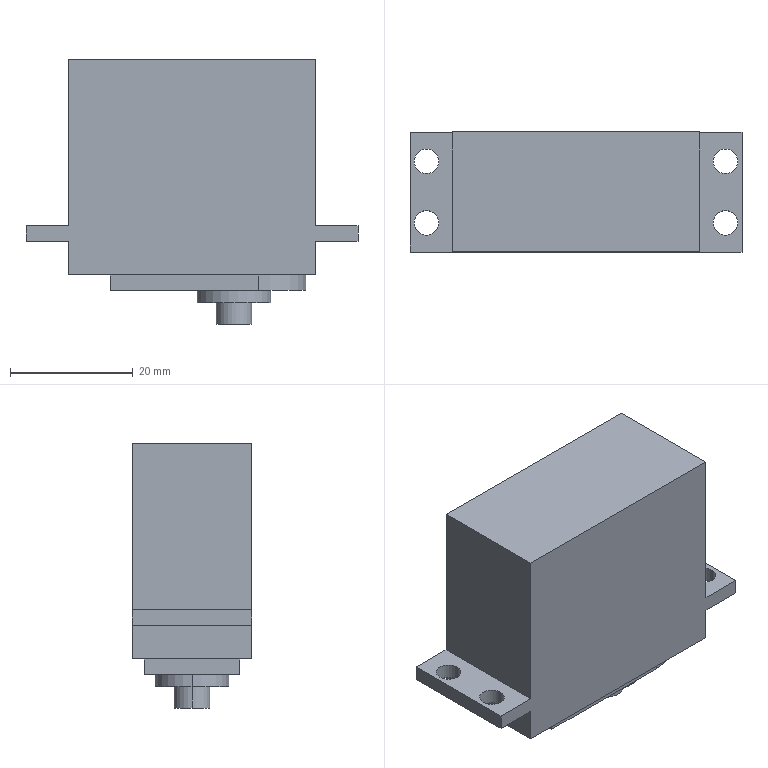Part | SolidWorks | features MBimport 1 | 2 solids | 43 faces | box 54 x 19.5 x 43 mm | volume 29172 mm3 | plane 24 | cylinder 19 | commonest cylinder face diameters 4 x8 3 x4 12 x4 5.8 x2 15.5 x1
STEP:
#1=CARTESIAN_POINT('',(-27.,9.75,0.));
#2=VERTEX_POINT('',#1);
#3=CARTESIAN_POINT('',(-27.,-9.75,0.));
#4=VERTEX_POINT('',#3);
#5=CARTESIAN_POINT('',(-27.,9.75,0.));
#6=DIRECTION('',(0.,-1.,0.));
#7=VECTOR('',#6,1000.);
#8=LINE('',#5,#7);
#9=EDGE_CURVE('',#2,#4,#8,.T.);
#10=ORIENTED_EDGE('',*,*,#9,.T.);
#11=CARTESIAN_POINT('',(-27.,-9.75,2.5));
#12=VERTEX_POINT('',#11);
#13=CARTESIAN_POINT('',(-27.,-9.75,0.));
#14=DIRECTION('',(0.,0.,1.));
#15=VECTOR('',#14,1000.);
#16=LINE('',#13,#15);
#17=EDGE_CURVE('',#4,#12,#16,.T.);
#18=ORIENTED_EDGE('',*,*,#17,.T.);
#19=CARTESIAN_POINT('',(-27.,9.75,2.5));
#20=VERTEX_POINT('',#19);
#21=CARTESIAN_POINT('',(-27.,9.75,2.5));
#22=DIRECTION('',(0.,-1.,0.));
#23=VECTOR('',#22,1000.);
#24=LINE('',#21,#23);
#25=EDGE_CURVE('',#20,#12,#24,.T.);
#26=ORIENTED_EDGE('',*,*,#25,.F.);
#27=CARTESIAN_POINT('',(-27.,9.75,0.));
#28=DIRECTION('',(0.,0.,1.));
#29=VECTOR('',#28,1000.);
#30=LINE('',#27,#29);
#31=EDGE_CURVE('',#2,#20,#30,.T.);
#32=ORIENTED_EDGE('',*,*,#31,.F.);
#33=EDGE_LOOP('',(#10,#18,#26,#32));
#34=FACE_OUTER_BOUND('',#33,.T.);
#35=CARTESIAN_POINT('',(-27.,9.75,0.));
#36=DIRECTION('',(-1.,0.,0.));
#37=DIRECTION('',(0.,0.,1.));
#38=AXIS2_PLACEMENT_3D('',#35,#36,#37);
#39=PLANE('',#38);
#40=ADVANCED_FACE('',(#34),#39,.T.);
#41=CARTESIAN_POINT('',(-26.315,5.,2.5));
#42=VERTEX_POINT('',#41);
#43=CARTESIAN_POINT('',(-26.315,5.,0.));
#44=VERTEX_POINT('',#43);
#45=CARTESIAN_POINT('',(-26.315,5.,2.5));
#46=DIRECTION('',(0.,0.,-1.));
#47=VECTOR('',#46,1000.);
#48=LINE('',#45,#47);
#49=EDGE_CURVE('',#42,#44,#48,.T.);
#50=ORIENTED_EDGE('',*,*,#49,.F.);
#51=CARTESIAN_POINT('',(-22.315,5.,2.5));
#52=VERTEX_POINT('',#51);
#53=CARTESIAN_POINT('',(-24.315,5.,2.5));
#54=DIRECTION('',(0.,0.,-1.));
#55=DIRECTION('',(1.,0.,0.));
#56=AXIS2_PLACEMENT_3D('',#53,#54,#55);
#57=CIRCLE('',#56,2.);
#58=EDGE_CURVE('',#52,#42,#57,.T.);
#59=ORIENTED_EDGE('',*,*,#58,.F.);
#60=CARTESIAN_POINT('',(-22.315,5.,0.));
#61=VERTEX_POINT('',#60);
#62=CARTESIAN_POINT('',(-22.315,5.,2.5));
#63=DIRECTION('',(0.,0.,-1.));
#64=VECTOR('',#63,1000.);
#65=LINE('',#62,#64);
#66=EDGE_CURVE('',#52,#61,#65,.T.);
#67=ORIENTED_EDGE('',*,*,#66,.T.);
#68=CARTESIAN_POINT('',(-24.315,5.,0.));
#69=DIRECTION('',(0.,0.,1.));
#70=DIRECTION('',(1.,0.,0.));
#71=AXIS2_PLACEMENT_3D('',#68,#69,#70);
#72=CIRCLE('',#71,2.);
#73=EDGE_CURVE('',#44,#61,#72,.T.);
#74=ORIENTED_EDGE('',*,*,#73,.F.);
#75=EDGE_LOOP('',(#50,#59,#67,#74));
#76=FACE_OUTER_BOUND('',#75,.T.);
#77=CARTESIAN_POINT('',(-24.315,5.,2.5));
#78=DIRECTION('',(0.,0.,-1.));
#79=DIRECTION('',(0.,1.,0.));
#80=AXIS2_PLACEMENT_3D('',#77,#78,#79);
#81=CYLINDRICAL_SURFACE('',#80,2.);
#82=ADVANCED_FACE('',(#76),#81,.F.);
#83=ORIENTED_EDGE('',*,*,#49,.T.);
#84=CARTESIAN_POINT('',(-24.315,5.,0.));
#85=DIRECTION('',(0.,0.,1.));
#86=DIRECTION('',(1.,0.,0.));
#87=AXIS2_PLACEMENT_3D('',#84,#85,#86);
#88=CIRCLE('',#87,2.);
#89=EDGE_CURVE('',#61,#44,#88,.T.);
#90=ORIENTED_EDGE('',*,*,#89,.F.);
#91=ORIENTED_EDGE('',*,*,#66,.F.);
#92=CARTESIAN_POINT('',(-24.315,5.,2.5));
#93=DIRECTION('',(0.,0.,-1.));
#94=DIRECTION('',(1.,0.,0.));
#95=AXIS2_PLACEMENT_3D('',#92,#93,#94);
#96=CIRCLE('',#95,2.);
#97=EDGE_CURVE('',#42,#52,#96,.T.);
#98=ORIENTED_EDGE('',*,*,#97,.F.);
#99=EDGE_LOOP('',(#83,#90,#91,#98));
#100=FACE_OUTER_BOUND('',#99,.T.);
#101=CARTESIAN_POINT('',(-24.315,5.,2.5));
#102=DIRECTION('',(0.,0.,-1.));
#103=DIRECTION('',(0.,-1.,0.));
#104=AXIS2_PLACEMENT_3D('',#101,#102,#103);
#105=CYLINDRICAL_SURFACE('',#104,2.);
#106=ADVANCED_FACE('',(#100),#105,.F.);
#107=CARTESIAN_POINT('',(-26.315,-5.,2.5));
#108=VERTEX_POINT('',#107);
#109=CARTESIAN_POINT('',(-26.315,-5.,0.));
#110=VERTEX_POINT('',#109);
#111=CARTESIAN_POINT('',(-26.315,-5.,2.5));
#112=DIRECTION('',(0.,0.,-1.));
#113=VECTOR('',#112,1000.);
#114=LINE('',#111,#113);
#115=EDGE_CURVE('',#108,#110,#114,.T.);
#116=ORIENTED_EDGE('',*,*,#115,.T.);
#117=CARTESIAN_POINT('',(-22.315,-5.,0.));
#118=VERTEX_POINT('',#117);
#119=CARTESIAN_POINT('',(-24.315,-5.,0.));
#120=DIRECTION('',(0.,0.,1.));
#121=DIRECTION('',(1.,0.,0.));
#122=AXIS2_PLACEMENT_3D('',#119,#120,#121);
#123=CIRCLE('',#122,2.);
#124=EDGE_CURVE('',#118,#110,#123,.T.);
#125=ORIENTED_EDGE('',*,*,#124,.F.);
#126=CARTESIAN_POINT('',(-22.315,-5.,2.5));
#127=VERTEX_POINT('',#126);
#128=CARTESIAN_POINT('',(-22.315,-5.,2.5));
#129=DIRECTION('',(0.,0.,-1.));
#130=VECTOR('',#129,1000.);
#131=LINE('',#128,#130);
#132=EDGE_CURVE('',#127,#118,#131,.T.);
#133=ORIENTED_EDGE('',*,*,#132,.F.);
#134=CARTESIAN_POINT('',(-24.315,-5.,2.5));
#135=DIRECTION('',(0.,0.,-1.));
#136=DIRECTION('',(1.,0.,0.));
#137=AXIS2_PLACEMENT_3D('',#134,#135,#136);
#138=CIRCLE('',#137,2.);
#139=EDGE_CURVE('',#108,#127,#138,.T.);
#140=ORIENTED_EDGE('',*,*,#139,.F.);
#141=EDGE_LOOP('',(#116,#125,#133,#140));
#142=FACE_OUTER_BOUND('',#141,.T.);
#143=CARTESIAN_POINT('',(-24.315,-5.,2.5));
#144=DIRECTION('',(0.,0.,-1.));
#145=DIRECTION('',(0.,-1.,0.));
#146=AXIS2_PLACEMENT_3D('',#143,#144,#145);
#147=CYLINDRICAL_SURFACE('',#146,2.);
#148=ADVANCED_FACE('',(#142),#147,.F.);
#149=CARTESIAN_POINT('',(-24.315,-5.,0.));
#150=DIRECTION('',(0.,0.,1.));
#151=DIRECTION('',(1.,0.,0.));
#152=AXIS2_PLACEMENT_3D('',#149,#150,#151);
#153=CIRCLE('',#152,2.);
#154=EDGE_CURVE('',#110,#118,#153,.T.);
#155=ORIENTED_EDGE('',*,*,#154,.T.);
#156=ORIENTED_EDGE('',*,*,#124,.T.);
#157=EDGE_LOOP('',(#155,#156));
#158=FACE_BOUND('',#157,.T.);
#159=ORIENTED_EDGE('',*,*,#73,.T.);
#160=ORIENTED_EDGE('',*,*,#89,.T.);
#161=EDGE_LOOP('',(#159,#160));
#162=FACE_BOUND('',#161,.T.);
#163=CARTESIAN_POINT('',(-20.15,9.75,0.));
#164=VERTEX_POINT('',#163);
#165=CARTESIAN_POINT('',(-20.15,-9.75,0.));
#166=VERTEX_POINT('',#165);
#167=CARTESIAN_POINT('',(-20.15,-4.875,0.));
#168=DIRECTION('',(0.,-1.,0.));
#169=VECTOR('',#168,1000.);
#170=LINE('',#167,#169);
#171=EDGE_CURVE('',#164,#166,#170,.T.);
#172=ORIENTED_EDGE('',*,*,#171,.T.);
#173=CARTESIAN_POINT('',(-27.,-9.75,0.));
#174=DIRECTION('',(1.,0.,0.));
#175=VECTOR('',#174,1000.);
#176=LINE('',#173,#175);
#177=EDGE_CURVE('',#4,#166,#176,.T.);
#178=ORIENTED_EDGE('',*,*,#177,.F.);
#179=ORIENTED_EDGE('',*,*,#9,.F.);
#180=CARTESIAN_POINT('',(27.,9.75,0.));
#181=DIRECTION('',(-1.,0.,0.));
#182=VECTOR('',#181,1000.);
#183=LINE('',#180,#182);
#184=EDGE_CURVE('',#164,#2,#183,.T.);
#185=ORIENTED_EDGE('',*,*,#184,.F.);
#186=EDGE_LOOP('',(#172,#178,#179,#185));
#187=FACE_OUTER_BOUND('',#186,.T.);
#188=CARTESIAN_POINT('',(0.,0.,0.));
#189=DIRECTION('',(0.,0.,1.));
#190=DIRECTION('',(1.,0.,0.));
#191=AXIS2_PLACEMENT_3D('',#188,#189,#190);
#192=PLANE('',#191);
#193=ADVANCED_FACE('',(#158,#162,#187),#192,.F.);
#194=ORIENTED_EDGE('',*,*,#115,.F.);
#195=CARTESIAN_POINT('',(-24.315,-5.,2.5));
#196=DIRECTION('',(0.,0.,-1.));
#197=DIRECTION('',(1.,0.,0.));
#198=AXIS2_PLACEMENT_3D('',#195,#196,#197);
#199=CIRCLE('',#198,2.);
#200=EDGE_CURVE('',#127,#108,#199,.T.);
#201=ORIENTED_EDGE('',*,*,#200,.F.);
#202=ORIENTED_EDGE('',*,*,#132,.T.);
#203=ORIENTED_EDGE('',*,*,#154,.F.);
#204=EDGE_LOOP('',(#194,#201,#202,#203));
#205=FACE_OUTER_BOUND('',#204,.T.);
#206=CARTESIAN_POINT('',(-24.315,-5.,2.5));
#207=DIRECTION('',(0.,0.,-1.));
#208=DIRECTION('',(0.,1.,0.));
#209=AXIS2_PLACEMENT_3D('',#206,#207,#208);
#210=CYLINDRICAL_SURFACE('',#209,2.);
#211=ADVANCED_FACE('',(#205),#210,.F.);
#212=ORIENTED_EDGE('',*,*,#139,.T.);
#213=ORIENTED_EDGE('',*,*,#200,.T.);
#214=EDGE_LOOP('',(#212,#213));
#215=FACE_BOUND('',#214,.T.);
#216=ORIENTED_EDGE('',*,*,#97,.T.);
#217=ORIENTED_EDGE('',*,*,#58,.T.);
#218=EDGE_LOOP('',(#216,#217));
#219=FACE_BOUND('',#218,.T.);
#220=CARTESIAN_POINT('',(-20.15,-9.75,2.5));
#221=VERTEX_POINT('',#220);
#222=CARTESIAN_POINT('',(-20.15,9.75,2.5));
#223=VERTEX_POINT('',#222);
#224=CARTESIAN_POINT('',(-20.15,4.875,2.5));
#225=DIRECTION('',(0.,1.,0.));
#226=VECTOR('',#225,1000.);
#227=LINE('',#224,#226);
#228=EDGE_CURVE('',#221,#223,#227,.T.);
#229=ORIENTED_EDGE('',*,*,#228,.T.);
#230=CARTESIAN_POINT('',(27.,9.75,2.5));
#231=DIRECTION('',(-1.,0.,0.));
#232=VECTOR('',#231,1000.);
#233=LINE('',#230,#232);
#234=EDGE_CURVE('',#223,#20,#233,.T.);
#235=ORIENTED_EDGE('',*,*,#234,.T.);
#236=ORIENTED_EDGE('',*,*,#25,.T.);
#237=CARTESIAN_POINT('',(-27.,-9.75,2.5));
#238=DIRECTION('',(1.,0.,0.));
#239=VECTOR('',#238,1000.);
#240=LINE('',#237,#239);
#241=EDGE_CURVE('',#12,#221,#240,.T.);
#242=ORIENTED_EDGE('',*,*,#241,.T.);
#243=EDGE_LOOP('',(#229,#235,#236,#242));
#244=FACE_OUTER_BOUND('',#243,.T.);
#245=CARTESIAN_POINT('',(0.,0.,2.5));
#246=DIRECTION('',(0.,0.,1.));
#247=DIRECTION('',(1.,0.,0.));
#248=AXIS2_PLACEMENT_3D('',#245,#246,#247);
#249=PLANE('',#248);
#250=ADVANCED_FACE('',(#215,#219,#244),#249,.T.);
#251=ORIENTED_EDGE('',*,*,#228,.F.);
#252=CARTESIAN_POINT('',(-20.15,-9.75,29.5));
#253=VERTEX_POINT('',#252);
#254=CARTESIAN_POINT('',(-20.15,-9.75,2.5));
#255=DIRECTION('',(0.,0.,1.));
#256=VECTOR('',#255,1000.);
#257=LINE('',#254,#256);
#258=EDGE_CURVE('',#221,#253,#257,.T.);
#259=ORIENTED_EDGE('',*,*,#258,.T.);
#260=CARTESIAN_POINT('',(-20.15,9.75,29.5));
#261=VERTEX_POINT('',#260);
#262=CARTESIAN_POINT('',(-20.15,9.75,29.5));
#263=DIRECTION('',(0.,-1.,0.));
#264=VECTOR('',#263,1000.);
#265=LINE('',#262,#264);
#266=EDGE_CURVE('',#261,#253,#265,.T.);
#267=ORIENTED_EDGE('',*,*,#266,.F.);
#268=CARTESIAN_POINT('',(-20.15,9.75,2.5));
#269=DIRECTION('',(0.,0.,1.));
#270=VECTOR('',#269,1000.);
#271=LINE('',#268,#270);
#272=EDGE_CURVE('',#223,#261,#271,.T.);
#273=ORIENTED_EDGE('',*,*,#272,.F.);
#274=EDGE_LOOP('',(#251,#259,#267,#273));
#275=FACE_OUTER_BOUND('',#274,.T.);
#276=CARTESIAN_POINT('',(-20.15,9.75,2.5));
#277=DIRECTION('',(-1.,0.,0.));
#278=DIRECTION('',(0.,0.,1.));
#279=AXIS2_PLACEMENT_3D('',#276,#277,#278);
#280=PLANE('',#279);
#281=ADVANCED_FACE('',(#275),#280,.T.);
#282=ORIENTED_EDGE('',*,*,#266,.T.);
#283=CARTESIAN_POINT('',(20.15,-9.75,29.5));
#284=VERTEX_POINT('',#283);
#285=CARTESIAN_POINT('',(-27.,-9.75,29.5));
#286=DIRECTION('',(1.,0.,0.));
#287=VECTOR('',#286,1000.);
#288=LINE('',#285,#287);
#289=EDGE_CURVE('',#253,#284,#288,.T.);
#290=ORIENTED_EDGE('',*,*,#289,.T.);
#291=CARTESIAN_POINT('',(20.15,9.75,29.5));
#292=VERTEX_POINT('',#291);
#293=CARTESIAN_POINT('',(20.15,-9.75,29.5));
#294=DIRECTION('',(0.,1.,0.));
#295=VECTOR('',#294,1000.);
#296=LINE('',#293,#295);
#297=EDGE_CURVE('',#284,#292,#296,.T.);
#298=ORIENTED_EDGE('',*,*,#297,.T.);
#299=CARTESIAN_POINT('',(27.,9.75,29.5));
#300=DIRECTION('',(-1.,0.,0.));
#301=VECTOR('',#300,1000.);
#302=LINE('',#299,#301);
#303=EDGE_CURVE('',#292,#261,#302,.T.);
#304=ORIENTED_EDGE('',*,*,#303,.T.);
#305=EDGE_LOOP('',(#282,#290,#298,#304));
#306=FACE_OUTER_BOUND('',#305,.T.);
#307=CARTESIAN_POINT('',(0.,0.,29.5));
#308=DIRECTION('',(0.,0.,1.));
#309=DIRECTION('',(1.,0.,0.));
#310=AXIS2_PLACEMENT_3D('',#307,#308,#309);
#311=PLANE('',#310);
#312=ADVANCED_FACE('',(#306),#311,.T.);
#313=CARTESIAN_POINT('',(27.,-9.75,0.));
#314=VERTEX_POINT('',#313);
#315=CARTESIAN_POINT('',(27.,9.75,0.));
#316=VERTEX_POINT('',#315);
#317=CARTESIAN_POINT('',(27.,-9.75,0.));
#318=DIRECTION('',(0.,1.,0.));
#319=VECTOR('',#318,1000.);
#320=LINE('',#317,#319);
#321=EDGE_CURVE('',#314,#316,#320,.T.);
#322=ORIENTED_EDGE('',*,*,#321,.T.);
#323=CARTESIAN_POINT('',(27.,9.75,2.5));
#324=VERTEX_POINT('',#323);
#325=CARTESIAN_POINT('',(27.,9.75,0.));
#326=DIRECTION('',(0.,0.,1.));
#327=VECTOR('',#326,1000.);
#328=LINE('',#325,#327);
#329=EDGE_CURVE('',#316,#324,#328,.T.);
#330=ORIENTED_EDGE('',*,*,#329,.T.);
#331=CARTESIAN_POINT('',(27.,-9.75,2.5));
#332=VERTEX_POINT('',#331);
#333=CARTESIAN_POINT('',(27.,-9.75,2.5));
#334=DIRECTION('',(0.,1.,0.));
#335=VECTOR('',#334,1000.);
#336=LINE('',#333,#335);
#337=EDGE_CURVE('',#332,#324,#336,.T.);
#338=ORIENTED_EDGE('',*,*,#337,.F.);
#339=CARTESIAN_POINT('',(27.,-9.75,0.));
#340=DIRECTION('',(0.,0.,1.));
#341=VECTOR('',#340,1000.);
#342=LINE('',#339,#341);
#343=EDGE_CURVE('',#314,#332,#342,.T.);
#344=ORIENTED_EDGE('',*,*,#343,.F.);
#345=EDGE_LOOP('',(#322,#330,#338,#344));
#346=FACE_OUTER_BOUND('',#345,.T.);
#347=CARTESIAN_POINT('',(27.,-9.75,0.));
#348=DIRECTION('',(1.,0.,0.));
#349=DIRECTION('',(0.,1.,0.));
#350=AXIS2_PLACEMENT_3D('',#347,#348,#349);
#351=PLANE('',#350);
#352=ADVANCED_FACE('',(#346),#351,.T.);
#353=CARTESIAN_POINT('',(22.315,-5.,2.5));
#354=VERTEX_POINT('',#353);
#355=CARTESIAN_POINT('',(22.315,-5.,0.));
#356=VERTEX_POINT('',#355);
#357=CARTESIAN_POINT('',(22.315,-5.,2.5));
#358=DIRECTION('',(0.,0.,-1.));
#359=VECTOR('',#358,1000.);
#360=LINE('',#357,#359);
#361=EDGE_CURVE('',#354,#356,#360,.T.);
#362=ORIENTED_EDGE('',*,*,#361,.T.);
#363=CARTESIAN_POINT('',(26.315,-5.,0.));
#364=VERTEX_POINT('',#363);
#365=CARTESIAN_POINT('',(24.315,-5.,0.));
#366=DIRECTION('',(0.,0.,1.));
#367=DIRECTION('',(1.,0.,0.));
#368=AXIS2_PLACEMENT_3D('',#365,#366,#367);
#369=CIRCLE('',#368,2.);
#370=EDGE_CURVE('',#364,#356,#369,.T.);
#371=ORIENTED_EDGE('',*,*,#370,.F.);
#372=CARTESIAN_POINT('',(26.315,-5.,2.5));
#373=VERTEX_POINT('',#372);
#374=CARTESIAN_POINT('',(26.315,-5.,2.5));
#375=DIRECTION('',(0.,0.,-1.));
#376=VECTOR('',#375,1000.);
#377=LINE('',#374,#376);
#378=EDGE_CURVE('',#373,#364,#377,.T.);
#379=ORIENTED_EDGE('',*,*,#378,.F.);
#380=CARTESIAN_POINT('',(24.315,-5.,2.5));
#381=DIRECTION('',(0.,0.,-1.));
#382=DIRECTION('',(1.,0.,0.));
#383=AXIS2_PLACEMENT_3D('',#380,#381,#382);
#384=CIRCLE('',#383,2.);
#385=EDGE_CURVE('',#354,#373,#384,.T.);
#386=ORIENTED_EDGE('',*,*,#385,.F.);
#387=EDGE_LOOP('',(#362,#371,#379,#386));
#388=FACE_OUTER_BOUND('',#387,.T.);
#389=CARTESIAN_POINT('',(24.315,-5.,2.5));
#390=DIRECTION('',(0.,0.,-1.));
#391=DIRECTION('',(0.,-1.,0.));
#392=AXIS2_PLACEMENT_3D('',#389,#390,#391);
#393=CYLINDRICAL_SURFACE('',#392,2.);
#394=ADVANCED_FACE('',(#388),#393,.F.);
#395=ORIENTED_EDGE('',*,*,#361,.F.);
#396=CARTESIAN_POINT('',(24.315,-5.,2.5));
#397=DIRECTION('',(0.,0.,-1.));
#398=DIRECTION('',(1.,0.,0.));
#399=AXIS2_PLACEMENT_3D('',#396,#397,#398);
#400=CIRCLE('',#399,2.);
#401=EDGE_CURVE('',#373,#354,#400,.T.);
#402=ORIENTED_EDGE('',*,*,#401,.F.);
#403=ORIENTED_EDGE('',*,*,#378,.T.);
#404=CARTESIAN_POINT('',(24.315,-5.,0.));
#405=DIRECTION('',(0.,0.,1.));
#406=DIRECTION('',(1.,0.,0.));
#407=AXIS2_PLACEMENT_3D('',#404,#405,#406);
#408=CIRCLE('',#407,2.);
#409=EDGE_CURVE('',#356,#364,#408,.T.);
#410=ORIENTED_EDGE('',*,*,#409,.F.);
#411=EDGE_LOOP('',(#395,#402,#403,#410));
#412=FACE_OUTER_BOUND('',#411,.T.);
#413=CARTESIAN_POINT('',(24.315,-5.,2.5));
#414=DIRECTION('',(0.,0.,-1.));
#415=DIRECTION('',(0.,1.,0.));
#416=AXIS2_PLACEMENT_3D('',#413,#414,#415);
#417=CYLINDRICAL_SURFACE('',#416,2.);
#418=ADVANCED_FACE('',(#412),#417,.F.);
#419=CARTESIAN_POINT('',(22.315,5.,2.5));
#420=VERTEX_POINT('',#419);
#421=CARTESIAN_POINT('',(22.315,5.,0.));
#422=VERTEX_POINT('',#421);
#423=CARTESIAN_POINT('',(22.315,5.,2.5));
#424=DIRECTION('',(0.,0.,-1.));
#425=VECTOR('',#424,1000.);
#426=LINE('',#423,#425);
#427=EDGE_CURVE('',#420,#422,#426,.T.);
#428=ORIENTED_EDGE('',*,*,#427,.F.);
#429=CARTESIAN_POINT('',(26.315,5.,2.5));
#430=VERTEX_POINT('',#429);
#431=CARTESIAN_POINT('',(24.315,5.,2.5));
#432=DIRECTION('',(0.,0.,-1.));
#433=DIRECTION('',(1.,0.,0.));
#434=AXIS2_PLACEMENT_3D('',#431,#432,#433);
#435=CIRCLE('',#434,2.);
#436=EDGE_CURVE('',#430,#420,#435,.T.);
#437=ORIENTED_EDGE('',*,*,#436,.F.);
#438=CARTESIAN_POINT('',(26.315,5.,0.));
#439=VERTEX_POINT('',#438);
#440=CARTESIAN_POINT('',(26.315,5.,2.5));
#441=DIRECTION('',(0.,0.,-1.));
#442=VECTOR('',#441,1000.);
#443=LINE('',#440,#442);
#444=EDGE_CURVE('',#430,#439,#443,.T.);
#445=ORIENTED_EDGE('',*,*,#444,.T.);
#446=CARTESIAN_POINT('',(24.315,5.,0.));
#447=DIRECTION('',(0.,0.,1.));
#448=DIRECTION('',(1.,0.,0.));
#449=AXIS2_PLACEMENT_3D('',#446,#447,#448);
#450=CIRCLE('',#449,2.);
#451=EDGE_CURVE('',#422,#439,#450,.T.);
#452=ORIENTED_EDGE('',*,*,#451,.F.);
#453=EDGE_LOOP('',(#428,#437,#445,#452));
#454=FACE_OUTER_BOUND('',#453,.T.);
#455=CARTESIAN_POINT('',(24.315,5.,2.5));
#456=DIRECTION('',(0.,0.,-1.));
#457=DIRECTION('',(0.,1.,0.));
#458=AXIS2_PLACEMENT_3D('',#455,#456,#457);
#459=CYLINDRICAL_SURFACE('',#458,2.);
#460=ADVANCED_FACE('',(#454),#459,.F.);
#461=CARTESIAN_POINT('',(24.315,5.,2.5));
#462=DIRECTION('',(0.,0.,-1.));
#463=DIRECTION('',(1.,0.,0.));
#464=AXIS2_PLACEMENT_3D('',#461,#462,#463);
#465=CIRCLE('',#464,2.);
#466=EDGE_CURVE('',#420,#430,#465,.T.);
#467=ORIENTED_EDGE('',*,*,#466,.T.);
#468=ORIENTED_EDGE('',*,*,#436,.T.);
#469=EDGE_LOOP('',(#467,#468));
#470=FACE_BOUND('',#469,.T.);
#471=ORIENTED_EDGE('',*,*,#385,.T.);
#472=ORIENTED_EDGE('',*,*,#401,.T.);
#473=EDGE_LOOP('',(#471,#472));
#474=FACE_BOUND('',#473,.T.);
#475=CARTESIAN_POINT('',(20.15,9.75,2.5));
#476=VERTEX_POINT('',#475);
#477=CARTESIAN_POINT('',(20.15,-9.75,2.5));
#478=VERTEX_POINT('',#477);
#479=CARTESIAN_POINT('',(20.15,-4.875,2.5));
#480=DIRECTION('',(0.,-1.,0.));
#481=VECTOR('',#480,1000.);
#482=LINE('',#479,#481);
#483=EDGE_CURVE('',#476,#478,#482,.T.);
#484=ORIENTED_EDGE('',*,*,#483,.T.);
#485=CARTESIAN_POINT('',(-27.,-9.75,2.5));
#486=DIRECTION('',(1.,0.,0.));
#487=VECTOR('',#486,1000.);
#488=LINE('',#485,#487);
#489=EDGE_CURVE('',#478,#332,#488,.T.);
#490=ORIENTED_EDGE('',*,*,#489,.T.);
#491=ORIENTED_EDGE('',*,*,#337,.T.);
#492=CARTESIAN_POINT('',(27.,9.75,2.5));
#493=DIRECTION('',(-1.,0.,0.));
#494=VECTOR('',#493,1000.);
#495=LINE('',#492,#494);
#496=EDGE_CURVE('',#324,#476,#495,.T.);
#497=ORIENTED_EDGE('',*,*,#496,.T.);
#498=EDGE_LOOP('',(#484,#490,#491,#497));
#499=FACE_OUTER_BOUND('',#498,.T.);
#500=CARTESIAN_POINT('',(0.,0.,2.5));
#501=DIRECTION('',(0.,0.,1.));
#502=DIRECTION('',(1.,0.,0.));
#503=AXIS2_PLACEMENT_3D('',#500,#501,#502);
#504=PLANE('',#503);
#505=ADVANCED_FACE('',(#470,#474,#499),#504,.T.);
#506=ORIENTED_EDGE('',*,*,#427,.T.);
#507=CARTESIAN_POINT('',(24.315,5.,0.));
#508=DIRECTION('',(0.,0.,1.));
#509=DIRECTION('',(1.,0.,0.));
#510=AXIS2_PLACEMENT_3D('',#507,#508,#509);
#511=CIRCLE('',#510,2.);
#512=EDGE_CURVE('',#439,#422,#511,.T.);
#513=ORIENTED_EDGE('',*,*,#512,.F.);
#514=ORIENTED_EDGE('',*,*,#444,.F.);
#515=ORIENTED_EDGE('',*,*,#466,.F.);
#516=EDGE_LOOP('',(#506,#513,#514,#515));
#517=FACE_OUTER_BOUND('',#516,.T.);
#518=CARTESIAN_POINT('',(24.315,5.,2.5));
#519=DIRECTION('',(0.,0.,-1.));
#520=DIRECTION('',(0.,-1.,0.));
#521=AXIS2_PLACEMENT_3D('',#518,#519,#520);
#522=CYLINDRICAL_SURFACE('',#521,2.);
#523=ADVANCED_FACE('',(#517),#522,.F.);
#524=ORIENTED_EDGE('',*,*,#451,.T.);
#525=ORIENTED_EDGE('',*,*,#512,.T.);
#526=EDGE_LOOP('',(#524,#525));
#527=FACE_BOUND('',#526,.T.);
#528=ORIENTED_EDGE('',*,*,#409,.T.);
#529=ORIENTED_EDGE('',*,*,#370,.T.);
#530=EDGE_LOOP('',(#528,#529));
#531=FACE_BOUND('',#530,.T.);
#532=CARTESIAN_POINT('',(20.15,-9.75,0.));
#533=VERTEX_POINT('',#532);
#534=CARTESIAN_POINT('',(20.15,9.75,0.));
#535=VERTEX_POINT('',#534);
#536=CARTESIAN_POINT('',(20.15,4.875,0.));
#537=DIRECTION('',(0.,1.,0.));
#538=VECTOR('',#537,1000.);
#539=LINE('',#536,#538);
#540=EDGE_CURVE('',#533,#535,#539,.T.);
#541=ORIENTED_EDGE('',*,*,#540,.T.);
#542=CARTESIAN_POINT('',(27.,9.75,0.));
#543=DIRECTION('',(-1.,0.,0.));
#544=VECTOR('',#543,1000.);
#545=LINE('',#542,#544);
#546=EDGE_CURVE('',#316,#535,#545,.T.);
#547=ORIENTED_EDGE('',*,*,#546,.F.);
#548=ORIENTED_EDGE('',*,*,#321,.F.);
#549=CARTESIAN_POINT('',(-27.,-9.75,0.));
#550=DIRECTION('',(1.,0.,0.));
#551=VECTOR('',#550,1000.);
#552=LINE('',#549,#551);
#553=EDGE_CURVE('',#533,#314,#552,.T.);
#554=ORIENTED_EDGE('',*,*,#553,.F.);
#555=EDGE_LOOP('',(#541,#547,#548,#554));
#556=FACE_OUTER_BOUND('',#555,.T.);
#557=CARTESIAN_POINT('',(0.,0.,0.));
#558=DIRECTION('',(0.,0.,1.));
#559=DIRECTION('',(1.,0.,0.));
#560=AXIS2_PLACEMENT_3D('',#557,#558,#559);
#561=PLANE('',#560);
#562=ADVANCED_FACE('',(#527,#531,#556),#561,.F.);
#563=CARTESIAN_POINT('',(20.15,-9.75,-5.5));
#564=VERTEX_POINT('',#563);
#565=CARTESIAN_POINT('',(20.15,9.75,-5.5));
#566=VERTEX_POINT('',#565);
#567=CARTESIAN_POINT('',(20.15,4.875,-5.5));
#568=DIRECTION('',(0.,1.,0.));
#569=VECTOR('',#568,1000.);
#570=LINE('',#567,#569);
#571=EDGE_CURVE('',#564,#566,#570,.T.);
#572=ORIENTED_EDGE('',*,*,#571,.T.);
#573=CARTESIAN_POINT('',(20.15,9.75,2.5));
#574=DIRECTION('',(0.,0.,-1.));
#575=VECTOR('',#574,1000.);
#576=LINE('',#573,#575);
#577=EDGE_CURVE('',#535,#566,#576,.T.);
#578=ORIENTED_EDGE('',*,*,#577,.F.);
#579=ORIENTED_EDGE('',*,*,#540,.F.);
#580=CARTESIAN_POINT('',(20.15,-9.75,2.5));
#581=DIRECTION('',(0.,0.,-1.));
#582=VECTOR('',#581,1000.);
#583=LINE('',#580,#582);
#584=EDGE_CURVE('',#533,#564,#583,.T.);
#585=ORIENTED_EDGE('',*,*,#584,.T.);
#586=EDGE_LOOP('',(#572,#578,#579,#585));
#587=FACE_OUTER_BOUND('',#586,.T.);
#588=CARTESIAN_POINT('',(20.15,9.75,2.5));
#589=DIRECTION('',(1.,0.,0.));
#590=DIRECTION('',(0.,1.,0.));
#591=AXIS2_PLACEMENT_3D('',#588,#589,#590);
#592=PLANE('',#591);
#593=ADVANCED_FACE('',(#587),#592,.T.);
#594=CARTESIAN_POINT('',(-20.15,9.75,-5.5));
#595=VERTEX_POINT('',#594);
#596=CARTESIAN_POINT('',(20.15,9.75,-5.5));
#597=DIRECTION('',(1.,0.,0.));
#598=VECTOR('',#597,1000.);
#599=LINE('',#596,#598);
#600=EDGE_CURVE('',#595,#566,#599,.T.);
#601=ORIENTED_EDGE('',*,*,#600,.F.);
#602=CARTESIAN_POINT('',(-20.15,9.75,2.5));
#603=DIRECTION('',(0.,0.,-1.));
#604=VECTOR('',#603,1000.);
#605=LINE('',#602,#604);
#606=EDGE_CURVE('',#164,#595,#605,.T.);
#607=ORIENTED_EDGE('',*,*,#606,.F.);
#608=ORIENTED_EDGE('',*,*,#184,.T.);
#609=ORIENTED_EDGE('',*,*,#31,.T.);
#610=ORIENTED_EDGE('',*,*,#234,.F.);
#611=ORIENTED_EDGE('',*,*,#272,.T.);
#612=ORIENTED_EDGE('',*,*,#303,.F.);
#613=CARTESIAN_POINT('',(20.15,9.75,2.5));
#614=DIRECTION('',(0.,0.,1.));
#615=VECTOR('',#614,1000.);
#616=LINE('',#613,#615);
#617=EDGE_CURVE('',#476,#292,#616,.T.);
#618=ORIENTED_EDGE('',*,*,#617,.F.);
#619=ORIENTED_EDGE('',*,*,#496,.F.);
#620=ORIENTED_EDGE('',*,*,#329,.F.);
#621=ORIENTED_EDGE('',*,*,#546,.T.);
#622=ORIENTED_EDGE('',*,*,#577,.T.);
#623=EDGE_LOOP('',(#601,#607,#608,#609,#610,#611,#612,#618,#619,#620,#621,#622));
#624=FACE_OUTER_BOUND('',#623,.T.);
#625=CARTESIAN_POINT('',(27.,9.75,0.));
#626=DIRECTION('',(0.,1.,0.));
#627=DIRECTION('',(1.,0.,0.));
#628=AXIS2_PLACEMENT_3D('',#625,#626,#627);
#629=PLANE('',#628);
#630=ADVANCED_FACE('',(#624),#629,.T.);
#631=CARTESIAN_POINT('',(5.665,0.,2.5));
#632=VERTEX_POINT('',#631);
#633=CARTESIAN_POINT('',(5.665,0.,-5.5));
#634=VERTEX_POINT('',#633);
#635=CARTESIAN_POINT('',(5.665,0.,2.5));
#636=DIRECTION('',(0.,0.,-1.));
#637=VECTOR('',#636,1000.);
#638=LINE('',#635,#637);
#639=EDGE_CURVE('',#632,#634,#638,.T.);
#640=ORIENTED_EDGE('',*,*,#639,.F.);
#641=CARTESIAN_POINT('',(8.665,0.,2.5));
#642=VERTEX_POINT('',#641);
#643=CARTESIAN_POINT('',(7.165,0.,2.5));
#644=DIRECTION('',(0.,0.,-1.));
#645=DIRECTION('',(1.,0.,0.));
#646=AXIS2_PLACEMENT_3D('',#643,#644,#645);
#647=CIRCLE('',#646,1.5);
#648=EDGE_CURVE('',#642,#632,#647,.T.);
#649=ORIENTED_EDGE('',*,*,#648,.F.);
#650=CARTESIAN_POINT('',(8.665,0.,-5.5));
#651=VERTEX_POINT('',#650);
#652=CARTESIAN_POINT('',(8.665,0.,2.5));
#653=DIRECTION('',(0.,0.,-1.));
#654=VECTOR('',#653,1000.);
#655=LINE('',#652,#654);
#656=EDGE_CURVE('',#642,#651,#655,.T.);
#657=ORIENTED_EDGE('',*,*,#656,.T.);
#658=CARTESIAN_POINT('',(7.165,0.,-5.5));
#659=DIRECTION('',(0.,0.,1.));
#660=DIRECTION('',(1.,0.,0.));
#661=AXIS2_PLACEMENT_3D('',#658,#659,#660);
#662=CIRCLE('',#661,1.5);
#663=EDGE_CURVE('',#634,#651,#662,.T.);
#664=ORIENTED_EDGE('',*,*,#663,.F.);
#665=EDGE_LOOP('',(#640,#649,#657,#664));
#666=FACE_OUTER_BOUND('',#665,.T.);
#667=CARTESIAN_POINT('',(7.165,0.,2.5));
#668=DIRECTION('',(0.,0.,-1.));
#669=DIRECTION('',(0.,1.,0.));
#670=AXIS2_PLACEMENT_3D('',#667,#668,#669);
#671=CYLINDRICAL_SURFACE('',#670,1.5);
#672=ADVANCED_FACE('',(#666),#671,.F.);
#673=CARTESIAN_POINT('',(7.165,0.,2.5));
#674=DIRECTION('',(0.,0.,-1.));
#675=DIRECTION('',(1.,0.,0.));
#676=AXIS2_PLACEMENT_3D('',#673,#674,#675);
#677=CIRCLE('',#676,1.5);
#678=EDGE_CURVE('',#632,#642,#677,.T.);
#679=ORIENTED_EDGE('',*,*,#678,.T.);
#680=ORIENTED_EDGE('',*,*,#648,.T.);
#681=EDGE_LOOP('',(#679,#680));
#682=FACE_OUTER_BOUND('',#681,.T.);
#683=CARTESIAN_POINT('',(0.,0.,2.5));
#684=DIRECTION('',(0.,0.,1.));
#685=DIRECTION('',(1.,0.,0.));
#686=AXIS2_PLACEMENT_3D('',#683,#684,#685);
#687=PLANE('',#686);
#688=ADVANCED_FACE('',(#682),#687,.F.);
#689=ORIENTED_EDGE('',*,*,#639,.T.);
#690=CARTESIAN_POINT('',(7.165,0.,-5.5));
#691=DIRECTION('',(0.,0.,1.));
#692=DIRECTION('',(1.,0.,0.));
#693=AXIS2_PLACEMENT_3D('',#690,#691,#692);
#694=CIRCLE('',#693,1.5);
#695=EDGE_CURVE('',#651,#634,#694,.T.);
#696=ORIENTED_EDGE('',*,*,#695,.F.);
#697=ORIENTED_EDGE('',*,*,#656,.F.);
#698=ORIENTED_EDGE('',*,*,#678,.F.);
#699=EDGE_LOOP('',(#689,#696,#697,#698));
#700=FACE_OUTER_BOUND('',#699,.T.);
#701=CARTESIAN_POINT('',(7.165,0.,2.5));
#702=DIRECTION('',(0.,0.,-1.));
#703=DIRECTION('',(0.,-1.,0.));
#704=AXIS2_PLACEMENT_3D('',#701,#702,#703);
#705=CYLINDRICAL_SURFACE('',#704,1.5);
#706=ADVANCED_FACE('',(#700),#705,.F.);
#707=ORIENTED_EDGE('',*,*,#663,.T.);
#708=ORIENTED_EDGE('',*,*,#695,.T.);
#709=EDGE_LOOP('',(#707,#708));
#710=FACE_BOUND('',#709,.T.);
#711=CARTESIAN_POINT('',(0.815,0.,-5.5));
#712=VERTEX_POINT('',#711);
#713=CARTESIAN_POINT('',(12.815,0.,-5.5));
#714=VERTEX_POINT('',#713);
#715=CARTESIAN_POINT('',(6.815,0.,-5.5));
#716=DIRECTION('',(0.,0.,1.));
#717=DIRECTION('',(-1.,0.,0.));
#718=AXIS2_PLACEMENT_3D('',#715,#716,#717);
#719=CIRCLE('',#718,6.);
#720=EDGE_CURVE('',#712,#714,#719,.T.);
#721=ORIENTED_EDGE('',*,*,#720,.F.);
#722=CARTESIAN_POINT('',(6.815,0.,-5.5));
#723=DIRECTION('',(0.,0.,1.));
#724=DIRECTION('',(-1.,0.,0.));
#725=AXIS2_PLACEMENT_3D('',#722,#723,#724);
#726=CIRCLE('',#725,6.);
#727=EDGE_CURVE('',#714,#712,#726,.T.);
#728=ORIENTED_EDGE('',*,*,#727,.F.);
#729=EDGE_LOOP('',(#721,#728));
#730=FACE_OUTER_BOUND('',#729,.T.);
#731=CARTESIAN_POINT('',(3.425,0.,-5.5));
#732=DIRECTION('',(0.,0.,-1.));
#733=DIRECTION('',(0.,-1.,0.));
#734=AXIS2_PLACEMENT_3D('',#731,#732,#733);
#735=PLANE('',#734);
#736=ADVANCED_FACE('',(#710,#730),#735,.T.);
#737=CARTESIAN_POINT('',(12.815,0.,-8.));
#738=VERTEX_POINT('',#737);
#739=CARTESIAN_POINT('',(12.815,0.,-8.));
#740=DIRECTION('',(0.,0.,1.));
#741=VECTOR('',#740,1000.);
#742=LINE('',#739,#741);
#743=EDGE_CURVE('',#738,#714,#742,.T.);
#744=ORIENTED_EDGE('',*,*,#743,.F.);
#745=CARTESIAN_POINT('',(0.815,0.,-8.));
#746=VERTEX_POINT('',#745);
#747=CARTESIAN_POINT('',(6.815,0.,-8.));
#748=DIRECTION('',(0.,0.,-1.));
#749=DIRECTION('',(1.,0.,0.));
#750=AXIS2_PLACEMENT_3D('',#747,#748,#749);
#751=CIRCLE('',#750,6.);
#752=EDGE_CURVE('',#738,#746,#751,.T.);
#753=ORIENTED_EDGE('',*,*,#752,.T.);
#754=CARTESIAN_POINT('',(0.815,0.,-8.));
#755=DIRECTION('',(0.,0.,1.));
#756=VECTOR('',#755,1000.);
#757=LINE('',#754,#756);
#758=EDGE_CURVE('',#746,#712,#757,.T.);
#759=ORIENTED_EDGE('',*,*,#758,.T.);
#760=ORIENTED_EDGE('',*,*,#720,.T.);
#761=EDGE_LOOP('',(#744,#753,#759,#760));
#762=FACE_OUTER_BOUND('',#761,.T.);
#763=CARTESIAN_POINT('',(6.815,0.,-8.));
#764=DIRECTION('',(0.,0.,1.));
#765=DIRECTION('',(0.,1.,0.));
#766=AXIS2_PLACEMENT_3D('',#763,#764,#765);
#767=CYLINDRICAL_SURFACE('',#766,6.);
#768=ADVANCED_FACE('',(#762),#767,.F.);
#769=ORIENTED_EDGE('',*,*,#743,.T.);
#770=ORIENTED_EDGE('',*,*,#727,.T.);
#771=ORIENTED_EDGE('',*,*,#758,.F.);
#772=CARTESIAN_POINT('',(6.815,0.,-8.));
#773=DIRECTION('',(0.,0.,-1.));
#774=DIRECTION('',(1.,0.,0.));
#775=AXIS2_PLACEMENT_3D('',#772,#773,#774);
#776=CIRCLE('',#775,6.);
#777=EDGE_CURVE('',#746,#738,#776,.T.);
#778=ORIENTED_EDGE('',*,*,#777,.T.);
#779=EDGE_LOOP('',(#769,#770,#771,#778));
#780=FACE_OUTER_BOUND('',#779,.T.);
#781=CARTESIAN_POINT('',(6.815,0.,-8.));
#782=DIRECTION('',(0.,0.,1.));
#783=DIRECTION('',(0.,-1.,0.));
#784=AXIS2_PLACEMENT_3D('',#781,#782,#783);
#785=CYLINDRICAL_SURFACE('',#784,6.);
#786=ADVANCED_FACE('',(#780),#785,.F.);
#787=ORIENTED_EDGE('',*,*,#752,.F.);
#788=ORIENTED_EDGE('',*,*,#777,.F.);
#789=EDGE_LOOP('',(#787,#788));
#790=FACE_BOUND('',#789,.T.);
#791=CARTESIAN_POINT('',(10.815,7.75,-8.));
#792=VERTEX_POINT('',#791);
#793=CARTESIAN_POINT('',(10.815,-7.75,-8.));
#794=VERTEX_POINT('',#793);
#795=CARTESIAN_POINT('',(10.815,0.,-8.));
#796=DIRECTION('',(0.,0.,-1.));
#797=DIRECTION('',(1.,0.,0.));
#798=AXIS2_PLACEMENT_3D('',#795,#796,#797);
#799=CIRCLE('',#798,7.75);
#800=EDGE_CURVE('',#792,#794,#799,.T.);
#801=ORIENTED_EDGE('',*,*,#800,.T.);
#802=CARTESIAN_POINT('',(-13.3,-7.75,-8.));
#803=VERTEX_POINT('',#802);
#804=CARTESIAN_POINT('',(11.787,-7.75,-8.));
#805=DIRECTION('',(-1.,0.,0.));
#806=VECTOR('',#805,1000.);
#807=LINE('',#804,#806);
#808=EDGE_CURVE('',#794,#803,#807,.T.);
#809=ORIENTED_EDGE('',*,*,#808,.T.);
#810=CARTESIAN_POINT('',(-13.3,7.75,-8.));
#811=VERTEX_POINT('',#810);
#812=CARTESIAN_POINT('',(-13.3,-9.75,-8.));
#813=DIRECTION('',(0.,1.,0.));
#814=VECTOR('',#813,1000.);
#815=LINE('',#812,#814);
#816=EDGE_CURVE('',#803,#811,#815,.T.);
#817=ORIENTED_EDGE('',*,*,#816,.T.);
#818=CARTESIAN_POINT('',(-4.938,7.75,-8.));
#819=DIRECTION('',(1.,0.,0.));
#820=VECTOR('',#819,1000.);
#821=LINE('',#818,#820);
#822=EDGE_CURVE('',#811,#792,#821,.T.);
#823=ORIENTED_EDGE('',*,*,#822,.T.);
#824=EDGE_LOOP('',(#801,#809,#817,#823));
#825=FACE_OUTER_BOUND('',#824,.T.);
#826=CARTESIAN_POINT('',(3.425,0.,-8.));
#827=DIRECTION('',(0.,0.,-1.));
#828=DIRECTION('',(0.,-1.,0.));
#829=AXIS2_PLACEMENT_3D('',#826,#827,#828);
#830=PLANE('',#829);
#831=ADVANCED_FACE('',(#790,#825),#830,.T.);
#832=CARTESIAN_POINT('',(10.815,-7.75,-5.5));
#833=VERTEX_POINT('',#832);
#834=CARTESIAN_POINT('',(10.815,-7.75,-8.));
#835=DIRECTION('',(0.,0.,-1.));
#836=VECTOR('',#835,1000.);
#837=LINE('',#834,#836);
#838=EDGE_CURVE('',#833,#794,#837,.T.);
#839=ORIENTED_EDGE('',*,*,#838,.F.);
#840=CARTESIAN_POINT('',(-13.3,-7.75,-5.5));
#841=VERTEX_POINT('',#840);
#842=CARTESIAN_POINT('',(11.787,-7.75,-5.5));
#843=DIRECTION('',(-1.,0.,0.));
#844=VECTOR('',#843,1000.);
#845=LINE('',#842,#844);
#846=EDGE_CURVE('',#833,#841,#845,.T.);
#847=ORIENTED_EDGE('',*,*,#846,.T.);
#848=CARTESIAN_POINT('',(-13.3,-7.75,-6.75));
#849=DIRECTION('',(0.,0.,1.));
#850=VECTOR('',#849,1000.);
#851=LINE('',#848,#850);
#852=EDGE_CURVE('',#803,#841,#851,.T.);
#853=ORIENTED_EDGE('',*,*,#852,.F.);
#854=ORIENTED_EDGE('',*,*,#808,.F.);
#855=EDGE_LOOP('',(#839,#847,#853,#854));
#856=FACE_OUTER_BOUND('',#855,.T.);
#857=CARTESIAN_POINT('',(20.15,-7.75,-8.));
#858=DIRECTION('',(0.,1.,0.));
#859=DIRECTION('',(1.,0.,0.));
#860=AXIS2_PLACEMENT_3D('',#857,#858,#859);
#861=PLANE('',#860);
#862=ADVANCED_FACE('',(#856),#861,.F.);
#863=CARTESIAN_POINT('',(-13.3,7.75,-5.5));
#864=VERTEX_POINT('',#863);
#865=CARTESIAN_POINT('',(-13.3,7.75,-6.75));
#866=DIRECTION('',(0.,0.,-1.));
#867=VECTOR('',#866,1000.);
#868=LINE('',#865,#867);
#869=EDGE_CURVE('',#864,#811,#868,.T.);
#870=ORIENTED_EDGE('',*,*,#869,.T.);
#871=ORIENTED_EDGE('',*,*,#816,.F.);
#872=ORIENTED_EDGE('',*,*,#852,.T.);
#873=CARTESIAN_POINT('',(-13.3,-4.875,-5.5));
#874=DIRECTION('',(0.,-1.,0.));
#875=VECTOR('',#874,1000.);
#876=LINE('',#873,#875);
#877=EDGE_CURVE('',#864,#841,#876,.T.);
#878=ORIENTED_EDGE('',*,*,#877,.F.);
#879=EDGE_LOOP('',(#870,#871,#872,#878));
#880=FACE_OUTER_BOUND('',#879,.T.);
#881=CARTESIAN_POINT('',(-13.3,-9.75,-5.5));
#882=DIRECTION('',(-1.,0.,0.));
#883=DIRECTION('',(0.,0.,1.));
#884=AXIS2_PLACEMENT_3D('',#881,#882,#883);
#885=PLANE('',#884);
#886=ADVANCED_FACE('',(#880),#885,.T.);
#887=CARTESIAN_POINT('',(10.815,7.75,-5.5));
#888=VERTEX_POINT('',#887);
#889=CARTESIAN_POINT('',(10.815,7.75,-8.));
#890=DIRECTION('',(0.,0.,-1.));
#891=VECTOR('',#890,1000.);
#892=LINE('',#889,#891);
#893=EDGE_CURVE('',#888,#792,#892,.T.);
#894=ORIENTED_EDGE('',*,*,#893,.T.);
#895=ORIENTED_EDGE('',*,*,#822,.F.);
#896=ORIENTED_EDGE('',*,*,#869,.F.);
#897=CARTESIAN_POINT('',(-4.938,7.75,-5.5));
#898=DIRECTION('',(1.,0.,0.));
#899=VECTOR('',#898,1000.);
#900=LINE('',#897,#899);
#901=EDGE_CURVE('',#864,#888,#900,.T.);
#902=ORIENTED_EDGE('',*,*,#901,.T.);
#903=EDGE_LOOP('',(#894,#895,#896,#902));
#904=FACE_OUTER_BOUND('',#903,.T.);
#905=CARTESIAN_POINT('',(-13.3,7.75,-8.));
#906=DIRECTION('',(0.,-1.,0.));
#907=DIRECTION('',(0.,0.,-1.));
#908=AXIS2_PLACEMENT_3D('',#905,#906,#907);
#909=PLANE('',#908);
#910=ADVANCED_FACE('',(#904),#909,.F.);
#911=CARTESIAN_POINT('',(10.815,0.,-5.5));
#912=DIRECTION('',(0.,0.,-1.));
#913=DIRECTION('',(1.,0.,0.));
#914=AXIS2_PLACEMENT_3D('',#911,#912,#913);
#915=CIRCLE('',#914,7.75);
#916=EDGE_CURVE('',#888,#833,#915,.T.);
#917=ORIENTED_EDGE('',*,*,#916,.T.);
#918=ORIENTED_EDGE('',*,*,#838,.T.);
#919=ORIENTED_EDGE('',*,*,#800,.F.);
#920=ORIENTED_EDGE('',*,*,#893,.F.);
#921=EDGE_LOOP('',(#917,#918,#919,#920));
#922=FACE_OUTER_BOUND('',#921,.T.);
#923=CARTESIAN_POINT('',(10.815,0.,-8.));
#924=DIRECTION('',(0.,0.,1.));
#925=DIRECTION('',(-1.,0.,0.));
#926=AXIS2_PLACEMENT_3D('',#923,#924,#925);
#927=CYLINDRICAL_SURFACE('',#926,7.75);
#928=ADVANCED_FACE('',(#922),#927,.T.);
#929=ORIENTED_EDGE('',*,*,#901,.F.);
#930=ORIENTED_EDGE('',*,*,#877,.T.);
#931=ORIENTED_EDGE('',*,*,#846,.F.);
#932=ORIENTED_EDGE('',*,*,#916,.F.);
#933=EDGE_LOOP('',(#929,#930,#931,#932));
#934=FACE_BOUND('',#933,.T.);
#935=ORIENTED_EDGE('',*,*,#571,.F.);
#936=CARTESIAN_POINT('',(-20.15,-9.75,-5.5));
#937=VERTEX_POINT('',#936);
#938=CARTESIAN_POINT('',(-27.,-9.75,-5.5));
#939=DIRECTION('',(-1.,0.,0.));
#940=VECTOR('',#939,1000.);
#941=LINE('',#938,#940);
#942=EDGE_CURVE('',#564,#937,#941,.T.);
#943=ORIENTED_EDGE('',*,*,#942,.T.);
#944=CARTESIAN_POINT('',(-20.15,9.75,-5.5));
#945=DIRECTION('',(0.,1.,0.));
#946=VECTOR('',#945,1000.);
#947=LINE('',#944,#946);
#948=EDGE_CURVE('',#937,#595,#947,.T.);
#949=ORIENTED_EDGE('',*,*,#948,.T.);
#950=ORIENTED_EDGE('',*,*,#600,.T.);
#951=EDGE_LOOP('',(#935,#943,#949,#950));
#952=FACE_OUTER_BOUND('',#951,.T.);
#953=CARTESIAN_POINT('',(0.,0.,-5.5));
#954=DIRECTION('',(0.,0.,-1.));
#955=DIRECTION('',(0.,-1.,0.));
#956=AXIS2_PLACEMENT_3D('',#953,#954,#955);
#957=PLANE('',#956);
#958=ADVANCED_FACE('',(#934,#952),#957,.T.);
#959=ORIENTED_EDGE('',*,*,#171,.F.);
#960=ORIENTED_EDGE('',*,*,#606,.T.);
#961=ORIENTED_EDGE('',*,*,#948,.F.);
#962=CARTESIAN_POINT('',(-20.15,-9.75,2.5));
#963=DIRECTION('',(0.,0.,-1.));
#964=VECTOR('',#963,1000.);
#965=LINE('',#962,#964);
#966=EDGE_CURVE('',#166,#937,#965,.T.);
#967=ORIENTED_EDGE('',*,*,#966,.F.);
#968=EDGE_LOOP('',(#959,#960,#961,#967));
#969=FACE_OUTER_BOUND('',#968,.T.);
#970=CARTESIAN_POINT('',(-20.15,-9.75,2.5));
#971=DIRECTION('',(-1.,0.,0.));
#972=DIRECTION('',(0.,0.,1.));
#973=AXIS2_PLACEMENT_3D('',#970,#971,#972);
#974=PLANE('',#973);
#975=ADVANCED_FACE('',(#969),#974,.T.);
#976=ORIENTED_EDGE('',*,*,#942,.F.);
#977=ORIENTED_EDGE('',*,*,#584,.F.);
#978=ORIENTED_EDGE('',*,*,#553,.T.);
#979=ORIENTED_EDGE('',*,*,#343,.T.);
#980=ORIENTED_EDGE('',*,*,#489,.F.);
#981=CARTESIAN_POINT('',(20.15,-9.75,2.5));
#982=DIRECTION('',(0.,0.,1.));
#983=VECTOR('',#982,1000.);
#984=LINE('',#981,#983);
#985=EDGE_CURVE('',#478,#284,#984,.T.);
#986=ORIENTED_EDGE('',*,*,#985,.T.);
#987=ORIENTED_EDGE('',*,*,#289,.F.);
#988=ORIENTED_EDGE('',*,*,#258,.F.);
#989=ORIENTED_EDGE('',*,*,#241,.F.);
#990=ORIENTED_EDGE('',*,*,#17,.F.);
#991=ORIENTED_EDGE('',*,*,#177,.T.);
#992=ORIENTED_EDGE('',*,*,#966,.T.);
#993=EDGE_LOOP('',(#976,#977,#978,#979,#980,#986,#987,#988,#989,#990,#991,#992));
#994=FACE_OUTER_BOUND('',#993,.T.);
#995=CARTESIAN_POINT('',(-27.,-9.75,0.));
#996=DIRECTION('',(0.,-1.,0.));
#997=DIRECTION('',(-1.,0.,0.));
#998=AXIS2_PLACEMENT_3D('',#995,#996,#997);
#999=PLANE('',#998);
#1000=ADVANCED_FACE('',(#994),#999,.T.);
#1001=ORIENTED_EDGE('',*,*,#483,.F.);
#1002=ORIENTED_EDGE('',*,*,#617,.T.);
#1003=ORIENTED_EDGE('',*,*,#297,.F.);
#1004=ORIENTED_EDGE('',*,*,#985,.F.);
#1005=EDGE_LOOP('',(#1001,#1002,#1003,#1004));
#1006=FACE_OUTER_BOUND('',#1005,.T.);
#1007=CARTESIAN_POINT('',(20.15,-9.75,2.5));
#1008=DIRECTION('',(1.,0.,0.));
#1009=DIRECTION('',(0.,-1.,0.));
#1010=AXIS2_PLACEMENT_3D('',#1007,#1008,#1009);
#1011=PLANE('',#1010);
#1012=ADVANCED_FACE('',(#1006),#1011,.T.);
#1013=CLOSED_SHELL('',(#40,#82,#106,#148,#193,#211,#250,#281,#312,#352,#394,#418,#460,#505,#523,#562,#593,#630,#672,#688,#706,#736,#768,#786,#831,#862,#886,#910,#928,#958,#975,#1000,#1012));
#1014=MANIFOLD_SOLID_BREP('',#1013);
#1015=CARTESIAN_POINT('',(0.815,0.,-10.));
#1016=VERTEX_POINT('',#1015);
#1017=CARTESIAN_POINT('',(0.815,0.,-8.));
#1018=VERTEX_POINT('',#1017);
#1019=CARTESIAN_POINT('',(0.815,0.,-10.));
#1020=DIRECTION('',(0.,0.,1.));
#1021=VECTOR('',#1020,1000.);
#1022=LINE('',#1019,#1021);
#1023=EDGE_CURVE('',#1016,#1018,#1022,.T.);
#1024=ORIENTED_EDGE('',*,*,#1023,.T.);
#1025=CARTESIAN_POINT('',(12.815,0.,-8.));
#1026=VERTEX_POINT('',#1025);
#1027=CARTESIAN_POINT('',(6.815,0.,-8.));
#1028=DIRECTION('',(0.,0.,-1.));
#1029=DIRECTION('',(1.,0.,0.));
#1030=AXIS2_PLACEMENT_3D('',#1027,#1028,#1029);
#1031=CIRCLE('',#1030,6.);
#1032=EDGE_CURVE('',#1018,#1026,#1031,.T.);
#1033=ORIENTED_EDGE('',*,*,#1032,.T.);
#1034=CARTESIAN_POINT('',(12.815,0.,-10.));
#1035=VERTEX_POINT('',#1034);
#1036=CARTESIAN_POINT('',(12.815,0.,-10.));
#1037=DIRECTION('',(0.,0.,1.));
#1038=VECTOR('',#1037,1000.);
#1039=LINE('',#1036,#1038);
#1040=EDGE_CURVE('',#1035,#1026,#1039,.T.);
#1041=ORIENTED_EDGE('',*,*,#1040,.F.);
#1042=CARTESIAN_POINT('',(6.815,0.,-10.));
#1043=DIRECTION('',(0.,0.,-1.));
#1044=DIRECTION('',(1.,0.,0.));
#1045=AXIS2_PLACEMENT_3D('',#1042,#1043,#1044);
#1046=CIRCLE('',#1045,6.);
#1047=EDGE_CURVE('',#1016,#1035,#1046,.T.);
#1048=ORIENTED_EDGE('',*,*,#1047,.F.);
#1049=EDGE_LOOP('',(#1024,#1033,#1041,#1048));
#1050=FACE_OUTER_BOUND('',#1049,.T.);
#1051=CARTESIAN_POINT('',(6.815,0.,-10.));
#1052=DIRECTION('',(0.,0.,1.));
#1053=DIRECTION('',(0.,-1.,0.));
#1054=AXIS2_PLACEMENT_3D('',#1051,#1052,#1053);
#1055=CYLINDRICAL_SURFACE('',#1054,6.);
#1056=ADVANCED_FACE('',(#1050),#1055,.T.);
#1057=CARTESIAN_POINT('',(6.815,0.,-8.));
#1058=DIRECTION('',(0.,0.,-1.));
#1059=DIRECTION('',(1.,0.,0.));
#1060=AXIS2_PLACEMENT_3D('',#1057,#1058,#1059);
#1061=CIRCLE('',#1060,6.);
#1062=EDGE_CURVE('',#1026,#1018,#1061,.T.);
#1063=ORIENTED_EDGE('',*,*,#1062,.F.);
#1064=ORIENTED_EDGE('',*,*,#1032,.F.);
#1065=EDGE_LOOP('',(#1063,#1064));
#1066=FACE_OUTER_BOUND('',#1065,.T.);
#1067=CARTESIAN_POINT('',(6.815,0.,-8.));
#1068=DIRECTION('',(0.,0.,-1.));
#1069=DIRECTION('',(0.,-1.,0.));
#1070=AXIS2_PLACEMENT_3D('',#1067,#1068,#1069);
#1071=PLANE('',#1070);
#1072=ADVANCED_FACE('',(#1066),#1071,.F.);
#1073=ORIENTED_EDGE('',*,*,#1023,.F.);
#1074=CARTESIAN_POINT('',(6.815,0.,-10.));
#1075=DIRECTION('',(0.,0.,-1.));
#1076=DIRECTION('',(1.,0.,0.));
#1077=AXIS2_PLACEMENT_3D('',#1074,#1075,#1076);
#1078=CIRCLE('',#1077,6.);
#1079=EDGE_CURVE('',#1035,#1016,#1078,.T.);
#1080=ORIENTED_EDGE('',*,*,#1079,.F.);
#1081=ORIENTED_EDGE('',*,*,#1040,.T.);
#1082=ORIENTED_EDGE('',*,*,#1062,.T.);
#1083=EDGE_LOOP('',(#1073,#1080,#1081,#1082));
#1084=FACE_OUTER_BOUND('',#1083,.T.);
#1085=CARTESIAN_POINT('',(6.815,0.,-10.));
#1086=DIRECTION('',(0.,0.,1.));
#1087=DIRECTION('',(0.,1.,0.));
#1088=AXIS2_PLACEMENT_3D('',#1085,#1086,#1087);
#1089=CYLINDRICAL_SURFACE('',#1088,6.);
#1090=ADVANCED_FACE('',(#1084),#1089,.T.);
#1091=CARTESIAN_POINT('',(5.315,0.,-10.));
#1092=VERTEX_POINT('',#1091);
#1093=CARTESIAN_POINT('',(5.315,0.,-13.5));
#1094=VERTEX_POINT('',#1093);
#1095=CARTESIAN_POINT('',(5.315,0.,-10.));
#1096=DIRECTION('',(0.,0.,-1.));
#1097=VECTOR('',#1096,1000.);
#1098=LINE('',#1095,#1097);
#1099=EDGE_CURVE('',#1092,#1094,#1098,.T.);
#1100=ORIENTED_EDGE('',*,*,#1099,.F.);
#1101=CARTESIAN_POINT('',(8.315,0.,-10.));
#1102=VERTEX_POINT('',#1101);
#1103=CARTESIAN_POINT('',(6.815,0.,-10.));
#1104=DIRECTION('',(0.,0.,1.));
#1105=DIRECTION('',(1.,0.,0.));
#1106=AXIS2_PLACEMENT_3D('',#1103,#1104,#1105);
#1107=CIRCLE('',#1106,1.5);
#1108=EDGE_CURVE('',#1092,#1102,#1107,.T.);
#1109=ORIENTED_EDGE('',*,*,#1108,.T.);
#1110=CARTESIAN_POINT('',(8.315,0.,-13.5));
#1111=VERTEX_POINT('',#1110);
#1112=CARTESIAN_POINT('',(8.315,0.,-10.));
#1113=DIRECTION('',(0.,0.,-1.));
#1114=VECTOR('',#1113,1000.);
#1115=LINE('',#1112,#1114);
#1116=EDGE_CURVE('',#1102,#1111,#1115,.T.);
#1117=ORIENTED_EDGE('',*,*,#1116,.T.);
#1118=CARTESIAN_POINT('',(6.815,0.,-13.5));
#1119=DIRECTION('',(0.,0.,1.));
#1120=DIRECTION('',(1.,0.,0.));
#1121=AXIS2_PLACEMENT_3D('',#1118,#1119,#1120);
#1122=CIRCLE('',#1121,1.5);
#1123=EDGE_CURVE('',#1094,#1111,#1122,.T.);
#1124=ORIENTED_EDGE('',*,*,#1123,.F.);
#1125=EDGE_LOOP('',(#1100,#1109,#1117,#1124));
#1126=FACE_OUTER_BOUND('',#1125,.T.);
#1127=CARTESIAN_POINT('',(6.815,0.,-8.));
#1128=DIRECTION('',(0.,0.,-1.));
#1129=DIRECTION('',(0.,1.,0.));
#1130=AXIS2_PLACEMENT_3D('',#1127,#1128,#1129);
#1131=CYLINDRICAL_SURFACE('',#1130,1.5);
#1132=ADVANCED_FACE('',(#1126),#1131,.F.);
#1133=CARTESIAN_POINT('',(6.815,0.,-10.));
#1134=DIRECTION('',(0.,0.,1.));
#1135=DIRECTION('',(1.,0.,0.));
#1136=AXIS2_PLACEMENT_3D('',#1133,#1134,#1135);
#1137=CIRCLE('',#1136,1.5);
#1138=EDGE_CURVE('',#1102,#1092,#1137,.T.);
#1139=ORIENTED_EDGE('',*,*,#1138,.F.);
#1140=ORIENTED_EDGE('',*,*,#1108,.F.);
#1141=EDGE_LOOP('',(#1139,#1140));
#1142=FACE_OUTER_BOUND('',#1141,.T.);
#1143=CARTESIAN_POINT('',(6.815,0.,-10.));
#1144=DIRECTION('',(0.,0.,-1.));
#1145=DIRECTION('',(0.,-1.,0.));
#1146=AXIS2_PLACEMENT_3D('',#1143,#1144,#1145);
#1147=PLANE('',#1146);
#1148=ADVANCED_FACE('',(#1142),#1147,.T.);
#1149=ORIENTED_EDGE('',*,*,#1099,.T.);
#1150=CARTESIAN_POINT('',(6.815,0.,-13.5));
#1151=DIRECTION('',(0.,0.,1.));
#1152=DIRECTION('',(1.,0.,0.));
#1153=AXIS2_PLACEMENT_3D('',#1150,#1151,#1152);
#1154=CIRCLE('',#1153,1.5);
#1155=EDGE_CURVE('',#1111,#1094,#1154,.T.);
#1156=ORIENTED_EDGE('',*,*,#1155,.F.);
#1157=ORIENTED_EDGE('',*,*,#1116,.F.);
#1158=ORIENTED_EDGE('',*,*,#1138,.T.);
#1159=EDGE_LOOP('',(#1149,#1156,#1157,#1158));
#1160=FACE_OUTER_BOUND('',#1159,.T.);
#1161=CARTESIAN_POINT('',(6.815,0.,-8.));
#1162=DIRECTION('',(0.,0.,-1.));
#1163=DIRECTION('',(0.,-1.,0.));
#1164=AXIS2_PLACEMENT_3D('',#1161,#1162,#1163);
#1165=CYLINDRICAL_SURFACE('',#1164,1.5);
#1166=ADVANCED_FACE('',(#1160),#1165,.F.);
#1167=ORIENTED_EDGE('',*,*,#1123,.T.);
#1168=ORIENTED_EDGE('',*,*,#1155,.T.);
#1169=EDGE_LOOP('',(#1167,#1168));
#1170=FACE_BOUND('',#1169,.T.);
#1171=CARTESIAN_POINT('',(3.915,0.,-13.5));
#1172=VERTEX_POINT('',#1171);
#1173=CARTESIAN_POINT('',(9.715,0.,-13.5));
#1174=VERTEX_POINT('',#1173);
#1175=CARTESIAN_POINT('',(6.815,0.,-13.5));
#1176=DIRECTION('',(0.,0.,-1.));
#1177=DIRECTION('',(1.,0.,0.));
#1178=AXIS2_PLACEMENT_3D('',#1175,#1176,#1177);
#1179=CIRCLE('',#1178,2.9);
#1180=EDGE_CURVE('',#1172,#1174,#1179,.T.);
#1181=ORIENTED_EDGE('',*,*,#1180,.T.);
#1182=CARTESIAN_POINT('',(6.815,0.,-13.5));
#1183=DIRECTION('',(0.,0.,-1.));
#1184=DIRECTION('',(1.,0.,0.));
#1185=AXIS2_PLACEMENT_3D('',#1182,#1183,#1184);
#1186=CIRCLE('',#1185,2.9);
#1187=EDGE_CURVE('',#1174,#1172,#1186,.T.);
#1188=ORIENTED_EDGE('',*,*,#1187,.T.);
#1189=EDGE_LOOP('',(#1181,#1188));
#1190=FACE_OUTER_BOUND('',#1189,.T.);
#1191=CARTESIAN_POINT('',(6.815,0.,-13.5));
#1192=DIRECTION('',(0.,0.,-1.));
#1193=DIRECTION('',(0.,-1.,0.));
#1194=AXIS2_PLACEMENT_3D('',#1191,#1192,#1193);
#1195=PLANE('',#1194);
#1196=ADVANCED_FACE('',(#1170,#1190),#1195,.T.);
#1197=CARTESIAN_POINT('',(3.915,0.,-10.));
#1198=VERTEX_POINT('',#1197);
#1199=CARTESIAN_POINT('',(3.915,0.,-13.5));
#1200=DIRECTION('',(0.,0.,1.));
#1201=VECTOR('',#1200,1000.);
#1202=LINE('',#1199,#1201);
#1203=EDGE_CURVE('',#1172,#1198,#1202,.T.);
#1204=ORIENTED_EDGE('',*,*,#1203,.T.);
#1205=CARTESIAN_POINT('',(9.715,0.,-10.));
#1206=VERTEX_POINT('',#1205);
#1207=CARTESIAN_POINT('',(6.815,0.,-10.));
#1208=DIRECTION('',(0.,0.,-1.));
#1209=DIRECTION('',(1.,0.,0.));
#1210=AXIS2_PLACEMENT_3D('',#1207,#1208,#1209);
#1211=CIRCLE('',#1210,2.9);
#1212=EDGE_CURVE('',#1198,#1206,#1211,.T.);
#1213=ORIENTED_EDGE('',*,*,#1212,.T.);
#1214=CARTESIAN_POINT('',(9.715,0.,-13.5));
#1215=DIRECTION('',(0.,0.,1.));
#1216=VECTOR('',#1215,1000.);
#1217=LINE('',#1214,#1216);
#1218=EDGE_CURVE('',#1174,#1206,#1217,.T.);
#1219=ORIENTED_EDGE('',*,*,#1218,.F.);
#1220=ORIENTED_EDGE('',*,*,#1180,.F.);
#1221=EDGE_LOOP('',(#1204,#1213,#1219,#1220));
#1222=FACE_OUTER_BOUND('',#1221,.T.);
#1223=CARTESIAN_POINT('',(6.815,0.,-13.5));
#1224=DIRECTION('',(0.,0.,1.));
#1225=DIRECTION('',(0.,-1.,0.));
#1226=AXIS2_PLACEMENT_3D('',#1223,#1224,#1225);
#1227=CYLINDRICAL_SURFACE('',#1226,2.9);
#1228=ADVANCED_FACE('',(#1222),#1227,.T.);
#1229=CARTESIAN_POINT('',(6.815,0.,-10.));
#1230=DIRECTION('',(0.,0.,-1.));
#1231=DIRECTION('',(1.,0.,0.));
#1232=AXIS2_PLACEMENT_3D('',#1229,#1230,#1231);
#1233=CIRCLE('',#1232,2.9);
#1234=EDGE_CURVE('',#1206,#1198,#1233,.T.);
#1235=ORIENTED_EDGE('',*,*,#1234,.F.);
#1236=ORIENTED_EDGE('',*,*,#1212,.F.);
#1237=EDGE_LOOP('',(#1235,#1236));
#1238=FACE_BOUND('',#1237,.T.);
#1239=ORIENTED_EDGE('',*,*,#1047,.T.);
#1240=ORIENTED_EDGE('',*,*,#1079,.T.);
#1241=EDGE_LOOP('',(#1239,#1240));
#1242=FACE_OUTER_BOUND('',#1241,.T.);
#1243=CARTESIAN_POINT('',(6.815,0.,-10.));
#1244=DIRECTION('',(0.,0.,-1.));
#1245=DIRECTION('',(0.,-1.,0.));
#1246=AXIS2_PLACEMENT_3D('',#1243,#1244,#1245);
#1247=PLANE('',#1246);
#1248=ADVANCED_FACE('',(#1238,#1242),#1247,.T.);
#1249=ORIENTED_EDGE('',*,*,#1203,.F.);
#1250=ORIENTED_EDGE('',*,*,#1187,.F.);
#1251=ORIENTED_EDGE('',*,*,#1218,.T.);
#1252=ORIENTED_EDGE('',*,*,#1234,.T.);
#1253=EDGE_LOOP('',(#1249,#1250,#1251,#1252));
#1254=FACE_OUTER_BOUND('',#1253,.T.);
#1255=CARTESIAN_POINT('',(6.815,0.,-13.5));
#1256=DIRECTION('',(0.,0.,1.));
#1257=DIRECTION('',(0.,1.,0.));
#1258=AXIS2_PLACEMENT_3D('',#1255,#1256,#1257);
#1259=CYLINDRICAL_SURFACE('',#1258,2.9);
#1260=ADVANCED_FACE('',(#1254),#1259,.T.);
#1261=CLOSED_SHELL('',(#1056,#1072,#1090,#1132,#1148,#1166,#1196,#1228,#1248,#1260));
#1262=MANIFOLD_SOLID_BREP('',#1261);
#1263=CARTESIAN_POINT('',(0.,0.,0.));
#1264=DIRECTION('',(0.,0.,1.));
#1265=DIRECTION('',(1.,0.,0.));
#1266=AXIS2_PLACEMENT_3D('',#1263,#1264,#1265);
#1267=(LENGTH_UNIT()NAMED_UNIT(*)SI_UNIT(.MILLI.,.METRE.));
#1268=UNCERTAINTY_MEASURE_WITH_UNIT(LENGTH_MEASURE(0.00001),#1267,'','');
#1269=(NAMED_UNIT(*)PLANE_ANGLE_UNIT()SI_UNIT($,.RADIAN.));
#1270=(NAMED_UNIT(*)SI_UNIT($,.STERADIAN.)SOLID_ANGLE_UNIT());
#1271=(GEOMETRIC_REPRESENTATION_CONTEXT(3)GLOBAL_UNCERTAINTY_ASSIGNED_CONTEXT((#1268))GLOBAL_UNIT_ASSIGNED_CONTEXT((#1267,#1269,#1270))REPRESENTATION_CONTEXT('',''));
#1272=ADVANCED_BREP_SHAPE_REPRESENTATION('',(#1014,#1262,#1266),#1271);